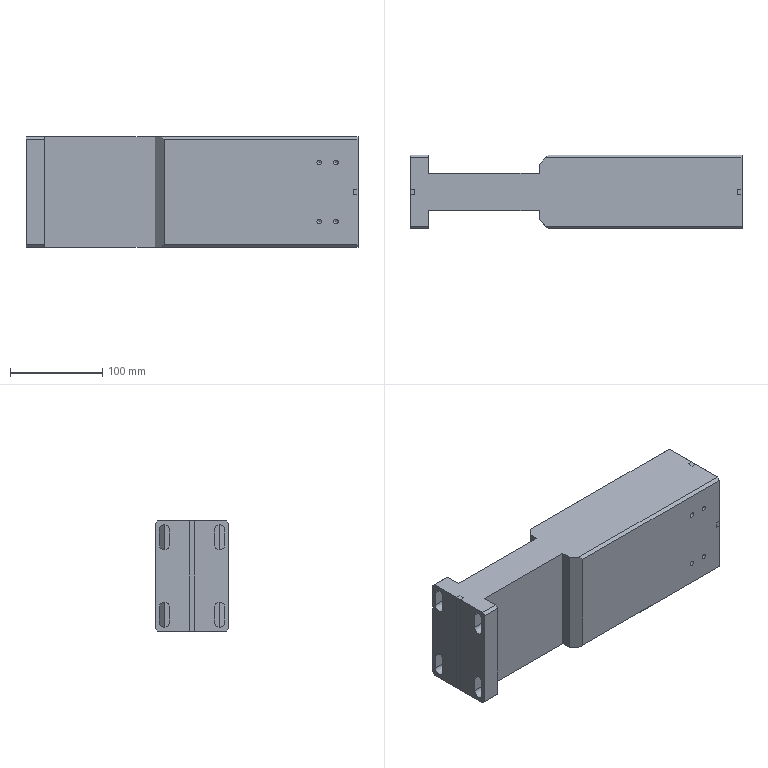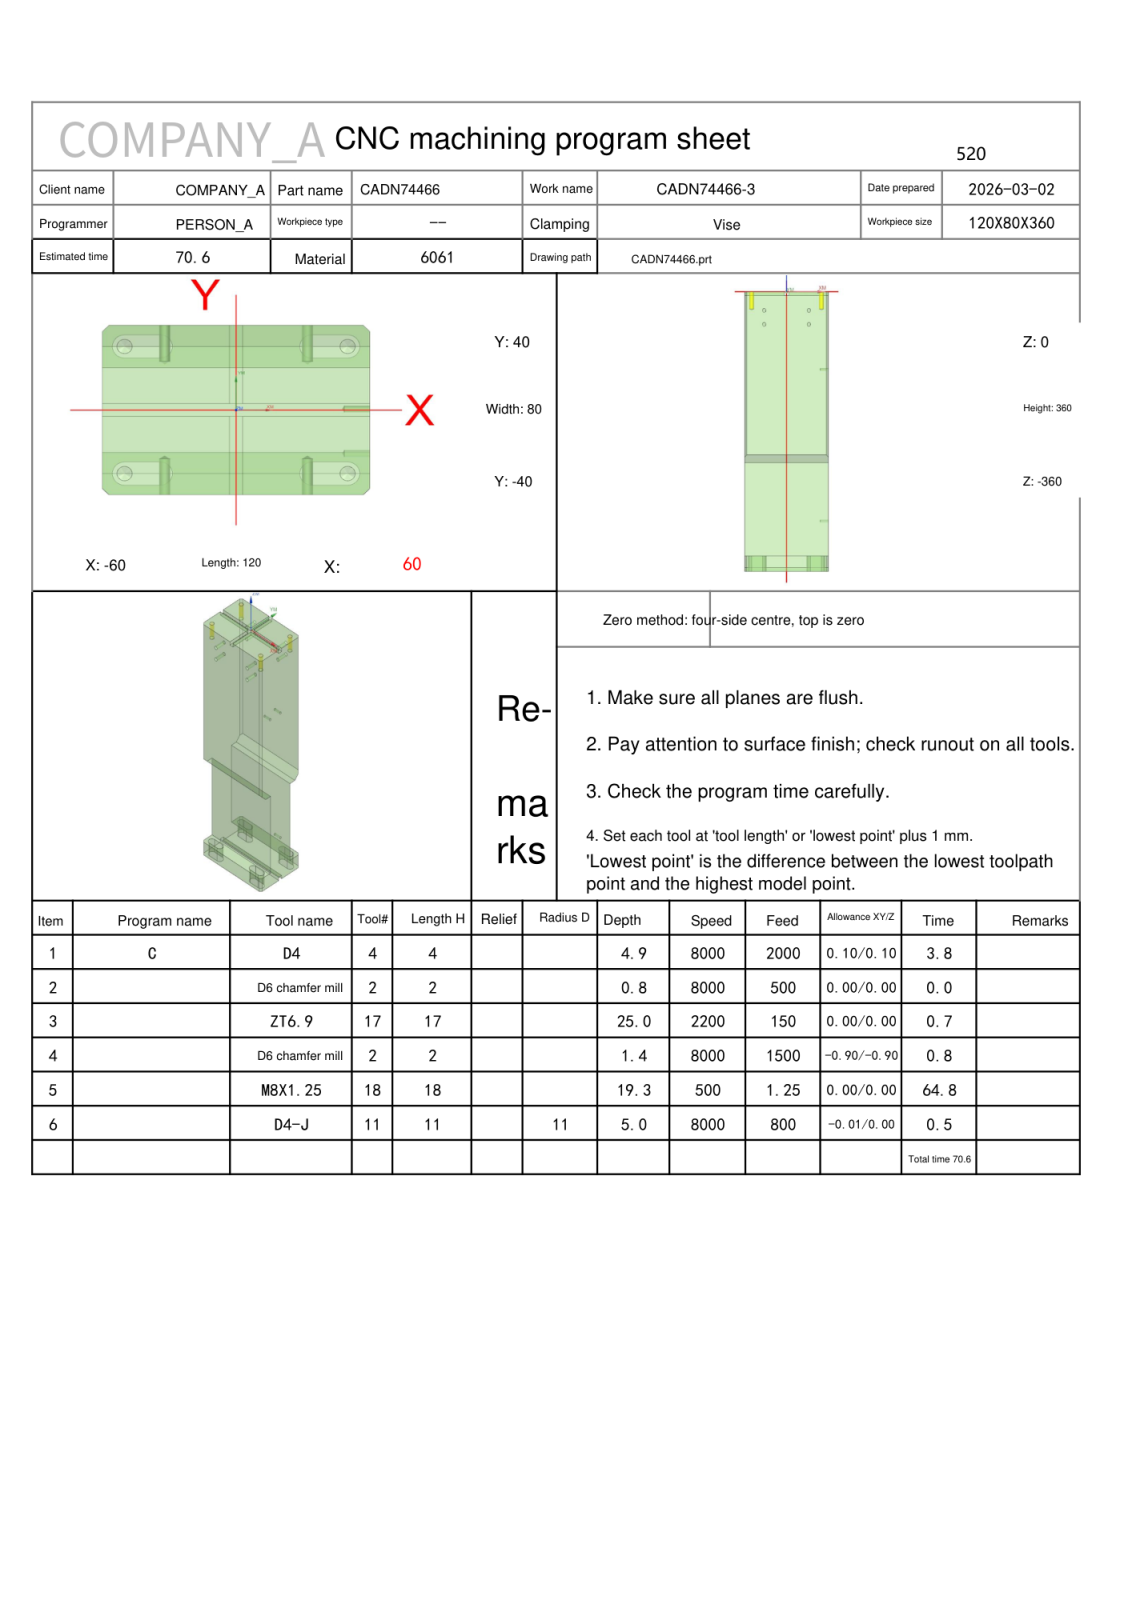NC program | NX | posted by the shop | part box 360 x 80 x 120 mm
Whole program:
%
O0001
(Machine time: 133.52 MIN)
(===Total Tool:5===)
(T4=D4      D=4.   R=0.   D-  H04 Z=-4.9  )
(T2=D6 chamfer mill   D=6.   R=0.   D-  H02 Z=-1.4  )
(T17=ZT6.9  D=6.9  DR_a=120 D-  H17 Z=-25.  )
(T18=M8X1.25 D=6.8  DR_a=180 D-  H18 Z=-19.25)
(T11=D4-J   D=4.   R=0.   D11 H11 Z=-5.   )
G80 G90 G17 G49 G40
G91 G28 Z0
M01
N1 T04 M06
(D4  D=4. R=0. H=04 ce=0.10 di=0.10)
G00 G90 G54 X65.1 Y.9 M03 S8000
G43 H04 Z10.1
M08
Z1.212
G01 Z-.288 F2000.
X61.96
X.9
Y41.96
Y45.1
Z1.212
G00 X-.9
G01 Z-.288
Y41.96
Y.9
X-61.96
X-65.1
Z1.212
G00 Y-.9
G01 Z-.288
X-61.96
X-.9
Y-41.96
Y-45.1
Z1.212
G00 X.9
G01 Z-.288
Y-41.96
Y-.9
X61.96
X65.1
Z1.212
G00 Y.9
Z.924
G01 Z-.576
X61.96
X.9
Y41.96
Y45.1
Z.924
G00 X-.9
G01 Z-.576
Y41.96
Y.9
X-61.96
X-65.1
Z.924
G00 Y-.9
G01 Z-.576
X-61.96
X-.9
Y-41.96
Y-45.1
Z.924
G00 X.9
G01 Z-.576
Y-41.96
Y-.9
X61.96
X65.1
Z.924
G00 Y.9
Z.635
G01 Z-.865
X61.96
X.9
Y41.96
Y45.1
Z.635
G00 X-.9
G01 Z-.865
Y41.96
Y.9
X-61.96
X-65.1
Z.635
G00 Y-.9
G01 Z-.865
X-61.96
X-.9
Y-41.96
Y-45.1
Z.635
G00 X.9
G01 Z-.865
Y-41.96
Y-.9
X61.96
X65.1
Z.635
G00 Y.9
Z.347
G01 Z-1.153
X61.96
X.9
Y41.96
Y45.1
Z.347
G00 X-.9
G01 Z-1.153
Y41.96
Y.9
X-61.96
X-65.1
Z.347
G00 Y-.9
G01 Z-1.153
X-61.96
X-.9
Y-41.96
Y-45.1
Z.347
G00 X.9
G01 Z-1.153
Y-41.96
Y-.9
X61.96
X65.1
Z.347
G00 Y.9
Z.059
G01 Z-1.441
X61.96
X.9
Y41.96
Y45.1
Z.059
G00 X-.9
G01 Z-1.441
Y41.96
Y.9
X-61.96
X-65.1
Z.059
G00 Y-.9
G01 Z-1.441
X-61.96
X-.9
Y-41.96
Y-45.1
Z.059
G00 X.9
G01 Z-1.441
Y-41.96
Y-.9
X61.96
X65.1
Z.059
G00 Y.9
Z-.229
G01 Z-1.729
X61.96
X.9
Y41.96
Y45.1
Z-.229
G00 X-.9
G01 Z-1.729
Y41.96
Y.9
X-61.96
X-65.1
Z-.229
G00 Y-.9
G01 Z-1.729
X-61.96
X-.9
Y-41.96
Y-45.1
Z-.229
G00 X.9
G01 Z-1.729
Y-41.96
Y-.9
X61.96
X65.1
Z-.229
G00 Y.9
Z-.518
G01 Z-2.018
X61.96
X.9
Y41.96
Y45.1
Z-.518
G00 X-.9
G01 Z-2.018
Y41.96
Y.9
X-61.96
X-65.1
Z-.518
G00 Y-.9
G01 Z-2.018
X-61.96
X-.9
Y-41.96
Y-45.1
Z-.518
G00 X.9
G01 Z-2.018
Y-41.96
Y-.9
X61.96
X65.1
Z-.518
G00 Y.9
Z-.806
G01 Z-2.306
X61.96
X.9
Y41.96
Y45.1
Z-.806
G00 X-.9
G01 Z-2.306
Y41.96
Y.9
X-61.96
X-65.1
Z-.806
G00 Y-.9
G01 Z-2.306
X-61.96
X-.9
Y-41.96
Y-45.1
Z-.806
G00 X.9
G01 Z-2.306
Y-41.96
Y-.9
X61.96
X65.1
Z-.806
G00 Y.9
Z-1.094
G01 Z-2.594
X61.96
X.9
Y41.96
Y45.1
Z-1.094
G00 X-.9
G01 Z-2.594
Y41.96
Y.9
X-61.96
X-65.1
Z-1.094
G00 Y-.9
G01 Z-2.594
X-61.96
X-.9
Y-41.96
Y-45.1
Z-1.094
G00 X.9
G01 Z-2.594
Y-41.96
Y-.9
X61.96
X65.1
Z-1.094
G00 Y.9
Z-1.382
G01 Z-2.882
X61.96
X.9
Y41.96
Y45.1
Z-1.382
G00 X-.9
G01 Z-2.882
Y41.96
Y.9
X-61.96
X-65.1
Z-1.382
G00 Y-.9
G01 Z-2.882
X-61.96
X-.9
Y-41.96
Y-45.1
Z-1.382
G00 X.9
G01 Z-2.882
Y-41.96
Y-.9
X61.96
X65.1
Z-1.382
G00 Y.9
Z-1.671
G01 Z-3.171
X61.96
X.9
Y41.96
Y45.1
Z-1.671
G00 X-.9
G01 Z-3.171
Y41.96
Y.9
X-61.96
X-65.1
Z-1.671
G00 Y-.9
G01 Z-3.171
X-61.96
X-.9
Y-41.96
Y-45.1
Z-1.671
G00 X.9
G01 Z-3.171
Y-41.96
Y-.9
X61.96
X65.1
Z-1.671
G00 Y.9
Z-1.959
G01 Z-3.459
X61.96
X.9
Y41.96
Y45.1
Z-1.959
G00 X-.9
G01 Z-3.459
Y41.96
Y.9
X-61.96
X-65.1
Z-1.959
G00 Y-.9
G01 Z-3.459
X-61.96
X-.9
Y-41.96
Y-45.1
Z-1.959
G00 X.9
G01 Z-3.459
Y-41.96
Y-.9
X61.96
X65.1
Z-1.959
G00 Y.9
Z-2.247
G01 Z-3.747
X61.96
X.9
Y41.96
Y45.1
Z-2.247
G00 X-.9
G01 Z-3.747
Y41.96
Y.9
X-61.96
X-65.1
Z-2.247
G00 Y-.9
G01 Z-3.747
X-61.96
X-.9
Y-41.96
Y-45.1
Z-2.247
G00 X.9
G01 Z-3.747
Y-41.96
Y-.9
X61.96
X65.1
Z-2.247
G00 Y.9
Z-2.535
G01 Z-4.035
X61.96
X.9
Y41.96
Y45.1
Z-2.535
G00 X-.9
G01 Z-4.035
Y41.96
Y.9
X-61.96
X-65.1
Z-2.535
G00 Y-.9
G01 Z-4.035
X-61.96
X-.9
Y-41.96
Y-45.1
Z-2.535
G00 X.9
G01 Z-4.035
Y-41.96
Y-.9
X61.96
X65.1
Z-2.535
G00 Y.9
Z-2.824
G01 Z-4.324
X61.96
X.9
Y41.96
Y45.1
Z-2.824
G00 X-.9
G01 Z-4.324
Y41.96
Y.9
X-61.96
X-65.1
Z-2.824
G00 Y-.9
G01 Z-4.324
X-61.96
X-.9
Y-41.96
Y-45.1
Z-2.824
G00 X.9
G01 Z-4.324
Y-41.96
Y-.9
X61.96
X65.1
Z-2.824
G00 Y.9
Z-3.112
G01 Z-4.612
X61.96
X.9
Y41.96
Y45.1
Z-3.112
G00 X-.9
G01 Z-4.612
Y41.96
Y.9
X-61.96
X-65.1
Z-3.112
G00 Y-.9
G01 Z-4.612
X-61.96
X-.9
Y-41.96
Y-45.1
Z-3.112
G00 X.9
G01 Z-4.612
Y-41.96
Y-.9
X61.96
X65.1
Z-3.112
G00 Y.9
Z-3.4
G01 Z-4.9
X61.96
X.9
Y41.96
Y45.1
Z-3.4
G00 X-.9
G01 Z-4.9
Y41.96
Y.9
X-61.96
X-65.1
Z-3.4
G00 Y-.9
G01 Z-4.9
X-61.96
X-.9
Y-41.96
Y-45.1
Z-3.4
G00 X.9
G01 Z-4.9
Y-41.96
Y-.9
X61.96
X65.1
Z-3.4
G00 Z10.1
G91 G28 Z0.0
M05
M09
G91 G28 Z0.0
M01
N2 T02 M06
(D6 chamfer mill  D=6. R=0. H=02 ce=0.00 di=0.10)
G00 G90 G54 X50. Y-30. M03 S8000
G43 H02 Z30.
M08
G98 G81 X50. Y-30. Z-.8 R1. F500.
Y30.
X-50.
Y-30.
G80
G00 Z30.
G91 G28 Z0.0
M05
M09
G91 G28 Z0.0
M01
N3 T17 M06
(ZT6.9 D=6.9 DR_a=120 H=17)
G00 G90 G54 X50. Y-30. M03 S2200
G43 H17 Z30.
M08
G98 G83 X50. Y-30. Z-25. R1. F150. Q2.
Y30.
X-50.
Y-30.
G80
G00 Z30.
G91 G28 Z0.0
M05
M09
G91 G28 Z0.0
M01
N4 T02 M06
(D6 chamfer mill  D=6. R=0. H=02 ce=-0.90 di=0.00)
G00 G90 G54 X-51.166 Y31.5 M03 S8000
G43 H02 Z30.
M08
Z-.9
G01 Z-1.4 F600.
X-51.4
G03 X-52.9 Y30. I0.0 J-1.5
X-50. Y27.1 I2.9 J0.0
X-47.1 Y30. I0.0 J2.9
X-50. Y32.9 I-2.9 J0.0
X-52.9 Y30. I0.0 J-2.9
X-51.4 Y28.5 I1.5 J0.0
G01 X-51.166
Z-.9
G00 Z30.
Y-28.5
Z-.9
G01 Z-1.4
X-51.4
G03 X-52.9 Y-30. I0.0 J-1.5
X-50. Y-32.9 I2.9 J0.0
X-47.1 Y-30. I0.0 J2.9
X-50. Y-27.1 I-2.9 J0.0
X-52.9 Y-30. I0.0 J-2.9
X-51.4 Y-31.5 I1.5 J0.0
G01 X-51.166
Z-.9
G00 Z30.
X48.834 Y-28.5
Z-.9
G01 Z-1.4
X48.6
G03 X47.1 Y-30. I0.0 J-1.5
X50. Y-32.9 I2.9 J0.0
X52.9 Y-30. I0.0 J2.9
X50. Y-27.1 I-2.9 J0.0
X47.1 Y-30. I0.0 J-2.9
X48.6 Y-31.5 I1.5 J0.0
G01 X48.834
Z-.9
G00 Z30.
Y31.5
Z-.9
G01 Z-1.4
X48.6
G03 X47.1 Y30. I0.0 J-1.5
X50. Y27.1 I2.9 J0.0
X52.9 Y30. I0.0 J2.9
X50. Y32.9 I-2.9 J0.0
X47.1 Y30. I0.0 J-2.9
X48.6 Y28.5 I1.5 J0.0
G01 X48.834
Z-.9
G00 Z30.
G00 G90 X-31.886 Y-1.773 M03 S6500
Z30.
Z.172
G01 Z-1.2 F1500.
G03 X-31.6 Y-1.973 I1.286 J1.532
G01 X-31.554 Y-2.003
X-31.5 Y-2.
X-3.
G02 X-2. Y-3. I0.0 J-1.
G01 Y-40.
G02 X-3. Y-41. I-1. J0.0
G01 X-57.
X-57.259 Y-40.966
X-57.5 Y-40.866
X-57.707 Y-40.707
X-60.707 Y-37.707
X-60.866 Y-37.5
X-60.966 Y-37.259
X-61. Y-37.
Y-3.
G02 X-60. Y-2. I1. J0.0
G01 X-31.5
X-31.446 Y-2.003
X-31.4 Y-1.973
G03 X-31.114 Y-1.773 I-1. J1.732
G01 Z.172
G00 Z10.
X-52.208 Y-29.596
Z.252
G01 Z-1.2
G03 X-52.382 Y-29.898 I1.638 J-1.147
G01 X-52.408 Y-29.946
X-52.4 Y-30.
G03 X-50. Y-32.4 I2.4 J0.0
X-47.6 Y-30. I0.0 J2.4
X-50. Y-27.6 I-2.4 J0.0
X-52.4 Y-30. I0.0 J-2.4
G01 X-52.408 Y-30.054
X-52.382 Y-30.102
G03 X-52.208 Y-30.404 I1.813 J.845
G01 Z.252
G00 Z10.
X-31.114 Y1.773
Z.172
G01 Z-1.2
G03 X-31.4 Y1.973 I-1.286 J-1.532
G01 X-31.446 Y2.003
X-31.5 Y2.
X-60.
G02 X-61. Y3. I0.0 J1.
G01 Y37.
X-60.966 Y37.259
X-60.866 Y37.5
X-60.707 Y37.707
X-57.707 Y40.707
X-57.5 Y40.866
X-57.259 Y40.966
X-57. Y41.
X-3.
G02 X-2. Y40. I0.0 J-1.
G01 Y3.
G02 X-3. Y2. I-1. J0.0
G01 X-31.5
X-31.554 Y2.003
X-31.6 Y1.973
G03 X-31.886 Y1.773 I1. J-1.732
G01 Z.172
G00 Z10.
X-52.208 Y30.404
Z.252
G01 Z-1.2
G03 X-52.382 Y30.102 I1.638 J-1.147
G01 X-52.408 Y30.054
X-52.4 Y30.
G03 X-50. Y27.6 I2.4 J0.0
X-47.6 Y30. I0.0 J2.4
X-50. Y32.4 I-2.4 J0.0
X-52.4 Y30. I0.0 J-2.4
G01 X-52.408 Y29.946
X-52.382 Y29.898
G03 X-52.208 Y29.596 I1.813 J.845
G01 Z.252
G00 Z10.
X31.886 Y1.773
Z.172
G01 Z-1.2
G03 X31.6 Y1.973 I-1.286 J-1.532
G01 X31.554 Y2.003
X31.5 Y2.
X3.
G02 X2. Y3. I0.0 J1.
G01 Y40.
G02 X3. Y41. I1. J0.0
G01 X57.
X57.259 Y40.966
X57.5 Y40.866
X57.707 Y40.707
X60.707 Y37.707
X60.866 Y37.5
X60.966 Y37.259
X61. Y37.
Y3.
G02 X60. Y2. I-1. J0.0
G01 X31.5
X31.446 Y2.003
X31.4 Y1.973
G03 X31.114 Y1.773 I1. J-1.732
G01 Z.172
G00 Z10.
X47.792 Y30.404
Z.252
G01 Z-1.2
G03 X47.618 Y30.102 I1.638 J-1.147
G01 X47.592 Y30.054
X47.6 Y30.
G03 X50. Y27.6 I2.4 J0.0
X52.4 Y30. I0.0 J2.4
X50. Y32.4 I-2.4 J0.0
X47.6 Y30. I0.0 J-2.4
G01 X47.592 Y29.946
X47.618 Y29.898
G03 X47.792 Y29.596 I1.813 J.845
G01 Z.252
G00 Z10.
X31.114 Y-1.773
Z.172
G01 Z-1.2
G03 X31.4 Y-1.973 I1.286 J1.532
G01 X31.446 Y-2.003
X31.5 Y-2.
X60.
G02 X61. Y-3. I0.0 J-1.
G01 Y-37.
X60.966 Y-37.259
X60.866 Y-37.5
X60.707 Y-37.707
X57.707 Y-40.707
X57.5 Y-40.866
X57.259 Y-40.966
X57. Y-41.
X3.
G02 X2. Y-40. I0.0 J1.
G01 Y-3.
G02 X3. Y-2. I1. J0.0
G01 X31.5
X31.554 Y-2.003
X31.6 Y-1.973
G03 X31.886 Y-1.773 I-1. J1.732
G01 Z.172
G00 Z10.
X47.792 Y-29.596
Z.252
G01 Z-1.2
G03 X47.618 Y-29.898 I1.638 J-1.147
G01 X47.592 Y-29.946
X47.6 Y-30.
G03 X50. Y-32.4 I2.4 J0.0
X52.4 Y-30. I0.0 J2.4
X50. Y-27.6 I-2.4 J0.0
X47.6 Y-30. I0.0 J-2.4
G01 X47.592 Y-30.054
X47.618 Y-30.102
G03 X47.792 Y-30.404 I1.813 J.845
G01 Z.252
G00 Z30.
G91 G28 Z0.0
M05
M09
G91 G28 Z0.0
M01
N5 T18 M06
(M8X1.25 D=6.8 DR_a=180 H=18)
G00 G90 G54 X50. Y-30. M03 S500
G43 H18 Z30.
M08
G95
G98 G84 X50. Y-30. Z-19.25 R1. F1.25 Q4.
Y30.
X-50.
Y-30.
G80
G94
G00 Z30.
G91 G28 Z0.0
M05
M09
G91 G28 Z0.0
M01
N6 T11 M06
(D4-J  D=4. R=0. H=11 ce=-0.01 di=0.00)
G00 G90 G54 X-62.824 Y-.173 M03 S8000
G43 H11 Z10.001
M08
Z-4.
G01 Z-5. F800.
G41 D11
X-62.785 Y-.369
G03 X-62. Y-1.015 I.785 J.154
G01 X-1.015
Y-42.
G03 X-.369 Y-42.785 I.8 J0.0
G01 G40 X-.173 Y-42.824
X.173
G41 D11
X.369 Y-42.785
G03 X1.015 Y-42. I-.154 J.785
G01 Y-1.015
X62.
G03 X62.785 Y-.369 I0.0 J.8
G01 G40 X62.824 Y-.173
Y.173
G41 D11
X62.785 Y.369
G03 X62. Y1.015 I-.785 J-.154
G01 X1.015
Y42.
G03 X.369 Y42.785 I-.8 J0.0
G01 G40 X.173 Y42.824
X-.173
G41 D11
X-.369 Y42.785
G03 X-1.015 Y42. I.154 J-.785
G01 Y1.015
X-62.
G03 X-62.785 Y.369 I0.0 J-.8
G01 G40 X-62.824 Y.173
Z-4.
G00 Z10.001
M05
M09
G91 G28 Z0.0
G91 G28 Y0.0
M30
%